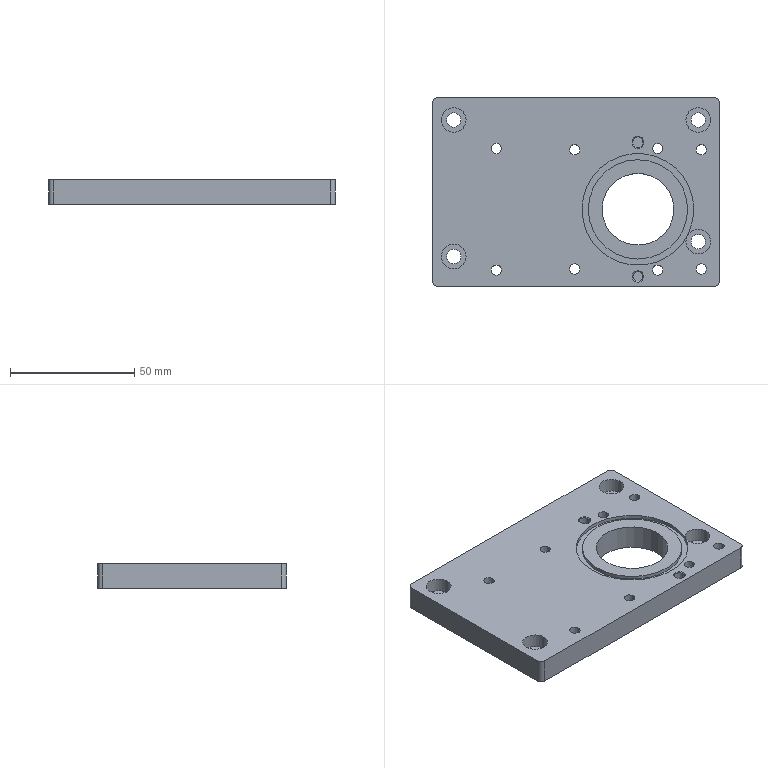Part | STEP file | 连接Plate 1 | 1 solid | 90 faces | box 115.5 x 76 x 10 mm | volume 76508 mm3 | cylinder 55 | plane 26 | cone 9 | commonest cylinder face diameters 4.134 x16 4 x8 5.8 x8 10 x8 5 x5 40 x4